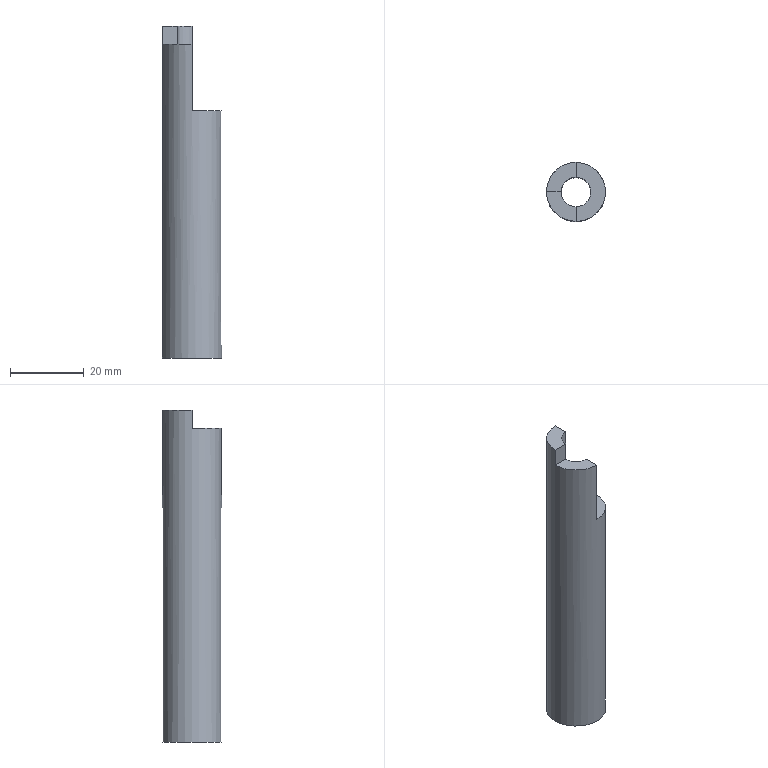Part | NX | features solid 2 | 1 solid | 9 faces | box 16 x 16 x 90 mm | volume 11646 mm3 | plane 7 | cylinder 2 | commonest cylinder face diameters 8.003 x1 16 x1
STEP:
#1=CARTESIAN_POINT('',(3418.699,-862.124,833.716));
#2=VERTEX_POINT('',#1);
#3=CARTESIAN_POINT('',(3418.699,-866.122,833.716));
#4=VERTEX_POINT('',#3);
#5=CARTESIAN_POINT('',(3418.699,-858.122,833.716));
#6=DIRECTION('',(0.,-1.,0.));
#7=VECTOR('',#6,1000.);
#8=LINE('',#5,#7);
#9=EDGE_CURVE('',#2,#4,#8,.T.);
#10=ORIENTED_EDGE('',*,*,#9,.T.);
#11=CARTESIAN_POINT('',(3418.699,-866.122,815.716));
#12=VERTEX_POINT('',#11);
#13=CARTESIAN_POINT('',(3418.699,-866.122,838.716));
#14=DIRECTION('',(0.,0.,-1.));
#15=VECTOR('',#14,1000.);
#16=LINE('',#13,#15);
#17=EDGE_CURVE('',#4,#12,#16,.T.);
#18=ORIENTED_EDGE('',*,*,#17,.T.);
#19=CARTESIAN_POINT('',(3418.699,-862.124,815.716));
#20=VERTEX_POINT('',#19);
#21=CARTESIAN_POINT('',(3418.699,-842.122,815.716));
#22=DIRECTION('',(0.,-1.,0.));
#23=VECTOR('',#22,1000.);
#24=LINE('',#21,#23);
#25=EDGE_CURVE('',#12,#20,#24,.F.);
#26=ORIENTED_EDGE('',*,*,#25,.T.);
#27=CARTESIAN_POINT('',(3418.699,-862.124,838.716));
#28=DIRECTION('',(0.,0.,-1.));
#29=VECTOR('',#28,1000.);
#30=LINE('',#27,#29);
#31=EDGE_CURVE('',#2,#20,#30,.T.);
#32=ORIENTED_EDGE('',*,*,#31,.F.);
#33=EDGE_LOOP('',(#10,#18,#26,#32));
#34=FACE_BOUND('',#33,.T.);
#35=CARTESIAN_POINT('',(3418.699,-842.122,815.716));
#36=DIRECTION('',(-1.,0.,0.));
#37=DIRECTION('',(0.,0.,1.));
#38=AXIS2_PLACEMENT_3D('',#35,#36,#37);
#39=PLANE('',#38);
#40=ADVANCED_FACE('',(#34),#39,.F.);
#41=CARTESIAN_POINT('',(3414.697,-858.122,748.716));
#42=VERTEX_POINT('',#41);
#43=CARTESIAN_POINT('',(3418.699,-858.122,748.716));
#44=DIRECTION('',(0.,0.,-1.));
#45=DIRECTION('',(-1.,0.,0.));
#46=AXIS2_PLACEMENT_3D('',#43,#44,#45);
#47=CIRCLE('',#46,4.002);
#48=EDGE_CURVE('',#42,#42,#47,.F.);
#49=ORIENTED_EDGE('',*,*,#48,.T.);
#50=EDGE_LOOP('',(#49));
#51=FACE_BOUND('',#50,.T.);
#52=CARTESIAN_POINT('',(3410.699,-858.122,748.716));
#53=VERTEX_POINT('',#52);
#54=CARTESIAN_POINT('',(3418.699,-858.122,748.716));
#55=DIRECTION('',(0.,0.,-1.));
#56=DIRECTION('',(-1.,0.,0.));
#57=AXIS2_PLACEMENT_3D('',#54,#55,#56);
#58=CIRCLE('',#57,8.);
#59=EDGE_CURVE('',#53,#53,#58,.F.);
#60=ORIENTED_EDGE('',*,*,#59,.F.);
#61=EDGE_LOOP('',(#60));
#62=FACE_BOUND('',#61,.T.);
#63=CARTESIAN_POINT('',(3418.699,-858.122,748.716));
#64=DIRECTION('',(0.,0.,-1.));
#65=DIRECTION('',(-1.,0.,0.));
#66=AXIS2_PLACEMENT_3D('',#63,#64,#65);
#67=PLANE('',#66);
#68=ADVANCED_FACE('',(#51,#62),#67,.T.);
#69=CARTESIAN_POINT('',(3414.697,-858.122,838.716));
#70=VERTEX_POINT('',#69);
#71=CARTESIAN_POINT('',(3410.699,-858.122,838.716));
#72=VERTEX_POINT('',#71);
#73=CARTESIAN_POINT('',(3418.699,-858.122,838.716));
#74=DIRECTION('',(-1.,0.,0.));
#75=VECTOR('',#74,1000.);
#76=LINE('',#73,#75);
#77=EDGE_CURVE('',#70,#72,#76,.T.);
#78=ORIENTED_EDGE('',*,*,#77,.F.);
#79=CARTESIAN_POINT('',(3418.699,-854.121,838.716));
#80=VERTEX_POINT('',#79);
#81=CARTESIAN_POINT('',(3418.699,-858.122,838.716));
#82=DIRECTION('',(0.,0.,-1.));
#83=DIRECTION('',(1.,0.,0.));
#84=AXIS2_PLACEMENT_3D('',#81,#82,#83);
#85=CIRCLE('',#84,4.002);
#86=EDGE_CURVE('',#70,#80,#85,.T.);
#87=ORIENTED_EDGE('',*,*,#86,.T.);
#88=CARTESIAN_POINT('',(3418.699,-850.122,838.716));
#89=VERTEX_POINT('',#88);
#90=CARTESIAN_POINT('',(3418.699,-842.122,838.716));
#91=DIRECTION('',(0.,-1.,0.));
#92=VECTOR('',#91,1000.);
#93=LINE('',#90,#92);
#94=EDGE_CURVE('',#89,#80,#93,.T.);
#95=ORIENTED_EDGE('',*,*,#94,.F.);
#96=CARTESIAN_POINT('',(3418.699,-858.122,838.716));
#97=DIRECTION('',(0.,0.,-1.));
#98=DIRECTION('',(1.,0.,0.));
#99=AXIS2_PLACEMENT_3D('',#96,#97,#98);
#100=CIRCLE('',#99,8.);
#101=EDGE_CURVE('',#72,#89,#100,.T.);
#102=ORIENTED_EDGE('',*,*,#101,.F.);
#103=EDGE_LOOP('',(#78,#87,#95,#102));
#104=FACE_BOUND('',#103,.T.);
#105=CARTESIAN_POINT('',(3418.699,-858.122,838.716));
#106=DIRECTION('',(0.,0.,1.));
#107=DIRECTION('',(1.,0.,0.));
#108=AXIS2_PLACEMENT_3D('',#105,#106,#107);
#109=PLANE('',#108);
#110=ADVANCED_FACE('',(#104),#109,.T.);
#111=CARTESIAN_POINT('',(3410.699,-858.122,833.716));
#112=VERTEX_POINT('',#111);
#113=CARTESIAN_POINT('',(3410.699,-858.122,838.716));
#114=DIRECTION('',(0.,0.,-1.));
#115=VECTOR('',#114,1000.);
#116=LINE('',#113,#115);
#117=EDGE_CURVE('',#72,#112,#116,.T.);
#118=ORIENTED_EDGE('',*,*,#117,.F.);
#119=ORIENTED_EDGE('',*,*,#101,.T.);
#120=CARTESIAN_POINT('',(3418.699,-850.122,815.716));
#121=VERTEX_POINT('',#120);
#122=CARTESIAN_POINT('',(3418.699,-850.122,838.716));
#123=DIRECTION('',(0.,0.,-1.));
#124=VECTOR('',#123,1000.);
#125=LINE('',#122,#124);
#126=EDGE_CURVE('',#121,#89,#125,.F.);
#127=ORIENTED_EDGE('',*,*,#126,.F.);
#128=CARTESIAN_POINT('',(3418.699,-858.122,815.716));
#129=DIRECTION('',(0.,0.,-1.));
#130=DIRECTION('',(-1.,0.,0.));
#131=AXIS2_PLACEMENT_3D('',#128,#129,#130);
#132=CIRCLE('',#131,8.);
#133=EDGE_CURVE('',#12,#121,#132,.F.);
#134=ORIENTED_EDGE('',*,*,#133,.F.);
#135=ORIENTED_EDGE('',*,*,#17,.F.);
#136=CARTESIAN_POINT('',(3418.699,-858.122,833.716));
#137=DIRECTION('',(0.,0.,1.));
#138=DIRECTION('',(1.,0.,0.));
#139=AXIS2_PLACEMENT_3D('',#136,#137,#138);
#140=CIRCLE('',#139,8.);
#141=EDGE_CURVE('',#4,#112,#140,.F.);
#142=ORIENTED_EDGE('',*,*,#141,.T.);
#143=EDGE_LOOP('',(#118,#119,#127,#134,#135,#142));
#144=FACE_BOUND('',#143,.T.);
#145=ORIENTED_EDGE('',*,*,#59,.T.);
#146=EDGE_LOOP('',(#145));
#147=FACE_BOUND('',#146,.T.);
#148=CARTESIAN_POINT('',(3418.699,-858.122,838.716));
#149=DIRECTION('',(0.,0.,-1.));
#150=DIRECTION('',(1.,0.,0.));
#151=AXIS2_PLACEMENT_3D('',#148,#149,#150);
#152=CYLINDRICAL_SURFACE('',#151,8.);
#153=ADVANCED_FACE('',(#144,#147),#152,.T.);
#154=ORIENTED_EDGE('',*,*,#48,.F.);
#155=EDGE_LOOP('',(#154));
#156=FACE_BOUND('',#155,.T.);
#157=ORIENTED_EDGE('',*,*,#86,.F.);
#158=CARTESIAN_POINT('',(3414.697,-858.122,833.716));
#159=VERTEX_POINT('',#158);
#160=CARTESIAN_POINT('',(3414.697,-858.122,838.716));
#161=DIRECTION('',(0.,0.,-1.));
#162=VECTOR('',#161,1000.);
#163=LINE('',#160,#162);
#164=EDGE_CURVE('',#70,#159,#163,.T.);
#165=ORIENTED_EDGE('',*,*,#164,.T.);
#166=CARTESIAN_POINT('',(3418.699,-858.122,833.716));
#167=DIRECTION('',(0.,0.,1.));
#168=DIRECTION('',(1.,0.,0.));
#169=AXIS2_PLACEMENT_3D('',#166,#167,#168);
#170=CIRCLE('',#169,4.002);
#171=EDGE_CURVE('',#2,#159,#170,.F.);
#172=ORIENTED_EDGE('',*,*,#171,.F.);
#173=ORIENTED_EDGE('',*,*,#31,.T.);
#174=CARTESIAN_POINT('',(3418.699,-854.121,815.716));
#175=VERTEX_POINT('',#174);
#176=CARTESIAN_POINT('',(3418.699,-858.122,815.716));
#177=DIRECTION('',(0.,0.,-1.));
#178=DIRECTION('',(-1.,0.,0.));
#179=AXIS2_PLACEMENT_3D('',#176,#177,#178);
#180=CIRCLE('',#179,4.002);
#181=EDGE_CURVE('',#20,#175,#180,.F.);
#182=ORIENTED_EDGE('',*,*,#181,.T.);
#183=CARTESIAN_POINT('',(3418.699,-854.121,838.716));
#184=DIRECTION('',(0.,0.,-1.));
#185=VECTOR('',#184,1000.);
#186=LINE('',#183,#185);
#187=EDGE_CURVE('',#175,#80,#186,.F.);
#188=ORIENTED_EDGE('',*,*,#187,.T.);
#189=EDGE_LOOP('',(#157,#165,#172,#173,#182,#188));
#190=FACE_BOUND('',#189,.T.);
#191=CARTESIAN_POINT('',(3418.699,-858.122,838.716));
#192=DIRECTION('',(0.,0.,-1.));
#193=DIRECTION('',(1.,0.,0.));
#194=AXIS2_PLACEMENT_3D('',#191,#192,#193);
#195=CYLINDRICAL_SURFACE('',#194,4.002);
#196=ADVANCED_FACE('',(#156,#190),#195,.F.);
#197=ORIENTED_EDGE('',*,*,#126,.T.);
#198=ORIENTED_EDGE('',*,*,#94,.T.);
#199=ORIENTED_EDGE('',*,*,#187,.F.);
#200=CARTESIAN_POINT('',(3418.699,-842.122,815.716));
#201=DIRECTION('',(0.,-1.,0.));
#202=VECTOR('',#201,1000.);
#203=LINE('',#200,#202);
#204=EDGE_CURVE('',#175,#121,#203,.F.);
#205=ORIENTED_EDGE('',*,*,#204,.T.);
#206=EDGE_LOOP('',(#197,#198,#199,#205));
#207=FACE_BOUND('',#206,.T.);
#208=CARTESIAN_POINT('',(3418.699,-842.122,815.716));
#209=DIRECTION('',(-1.,0.,0.));
#210=DIRECTION('',(0.,0.,1.));
#211=AXIS2_PLACEMENT_3D('',#208,#209,#210);
#212=PLANE('',#211);
#213=ADVANCED_FACE('',(#207),#212,.F.);
#214=ORIENTED_EDGE('',*,*,#133,.T.);
#215=ORIENTED_EDGE('',*,*,#204,.F.);
#216=ORIENTED_EDGE('',*,*,#181,.F.);
#217=ORIENTED_EDGE('',*,*,#25,.F.);
#218=EDGE_LOOP('',(#214,#215,#216,#217));
#219=FACE_BOUND('',#218,.T.);
#220=CARTESIAN_POINT('',(-438.,0.,815.716));
#221=DIRECTION('',(0.,0.,-1.));
#222=DIRECTION('',(-1.,0.,0.));
#223=AXIS2_PLACEMENT_3D('',#220,#221,#222);
#224=PLANE('',#223);
#225=ADVANCED_FACE('',(#219),#224,.F.);
#226=ORIENTED_EDGE('',*,*,#117,.T.);
#227=CARTESIAN_POINT('',(3418.699,-858.122,833.716));
#228=DIRECTION('',(-1.,0.,0.));
#229=VECTOR('',#228,1000.);
#230=LINE('',#227,#229);
#231=EDGE_CURVE('',#112,#159,#230,.F.);
#232=ORIENTED_EDGE('',*,*,#231,.T.);
#233=ORIENTED_EDGE('',*,*,#164,.F.);
#234=ORIENTED_EDGE('',*,*,#77,.T.);
#235=EDGE_LOOP('',(#226,#232,#233,#234));
#236=FACE_BOUND('',#235,.T.);
#237=CARTESIAN_POINT('',(3418.699,-858.122,833.716));
#238=DIRECTION('',(0.,1.,0.));
#239=DIRECTION('',(0.,0.,1.));
#240=AXIS2_PLACEMENT_3D('',#237,#238,#239);
#241=PLANE('',#240);
#242=ADVANCED_FACE('',(#236),#241,.F.);
#243=ORIENTED_EDGE('',*,*,#9,.F.);
#244=ORIENTED_EDGE('',*,*,#171,.T.);
#245=ORIENTED_EDGE('',*,*,#231,.F.);
#246=ORIENTED_EDGE('',*,*,#141,.F.);
#247=EDGE_LOOP('',(#243,#244,#245,#246));
#248=FACE_BOUND('',#247,.T.);
#249=CARTESIAN_POINT('',(-438.,0.,833.716));
#250=DIRECTION('',(0.,0.,1.));
#251=DIRECTION('',(1.,0.,0.));
#252=AXIS2_PLACEMENT_3D('',#249,#250,#251);
#253=PLANE('',#252);
#254=ADVANCED_FACE('',(#248),#253,.T.);
#255=CLOSED_SHELL('',(#40,#68,#110,#153,#196,#213,#225,#242,#254));
#256=MANIFOLD_SOLID_BREP('',#255);
#257=(LENGTH_UNIT()NAMED_UNIT(*)SI_UNIT(.MILLI.,.METRE.));
#258=UNCERTAINTY_MEASURE_WITH_UNIT(LENGTH_MEASURE(0.00001),#257,'','');
#259=(NAMED_UNIT(*)PLANE_ANGLE_UNIT()SI_UNIT($,.RADIAN.));
#260=(NAMED_UNIT(*)SI_UNIT($,.STERADIAN.)SOLID_ANGLE_UNIT());
#261=(GEOMETRIC_REPRESENTATION_CONTEXT(3)GLOBAL_UNCERTAINTY_ASSIGNED_CONTEXT((#258))GLOBAL_UNIT_ASSIGNED_CONTEXT((#257,#259,#260))REPRESENTATION_CONTEXT('',''));
#262=ADVANCED_BREP_SHAPE_REPRESENTATION('',(#256),#261);